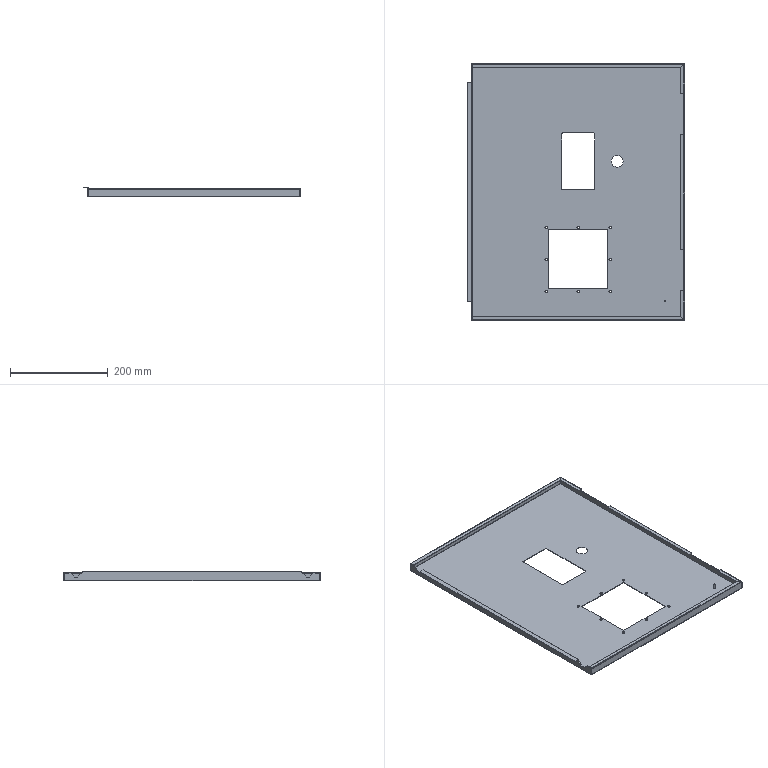Part | STEP file | left sheet-metal door panel | 1 solid | 161 faces | box 444.3 x 525.8 x 20.2 mm | volume 297154 mm3 | plane 105 | cylinder 50 | spline 6 | commonest cylinder face diameters 5 x16 0.02 x10 2.42 x10 4 x6 2 x4 3 x2